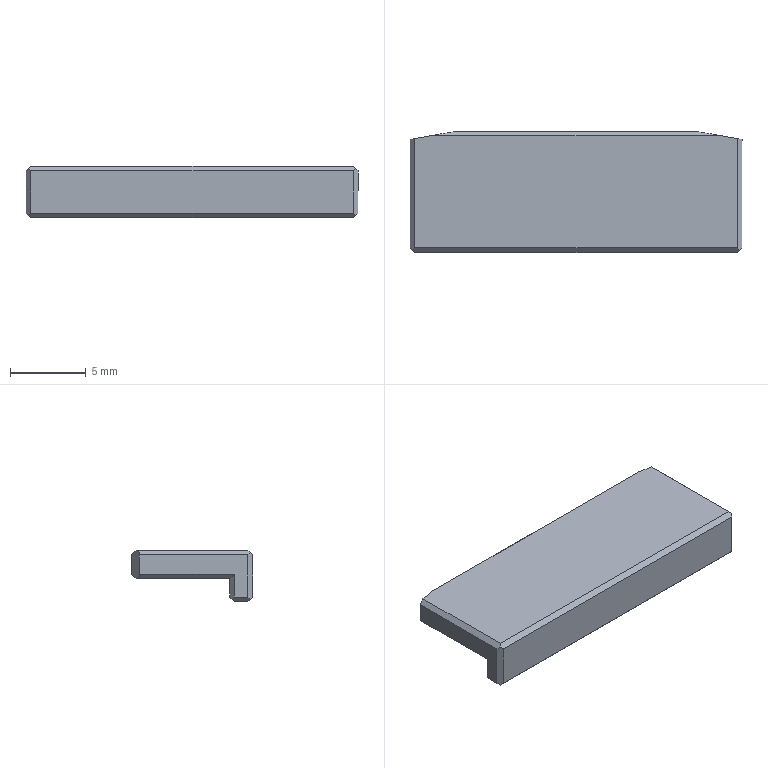Part | NX | 1 solid | 25 faces | box 21.95 x 8 x 3.38 mm | volume 370.348 mm3 | plane 25
STEP:
#1=CARTESIAN_POINT('',(-34.76,-62.629,7.853));
#2=VERTEX_POINT('',#1);
#3=CARTESIAN_POINT('',(-34.76,-56.605,7.853));
#4=VERTEX_POINT('',#3);
#5=CARTESIAN_POINT('',(-34.76,-59.529,7.853));
#6=DIRECTION('',(0.,1.,0.));
#7=VECTOR('',#6,1000.);
#8=LINE('',#5,#7);
#9=EDGE_CURVE('',#2,#4,#8,.T.);
#10=ORIENTED_EDGE('',*,*,#9,.T.);
#11=CARTESIAN_POINT('',(-33.762,-56.429,7.853));
#12=VERTEX_POINT('',#11);
#13=CARTESIAN_POINT('',(-22.513,-54.446,7.853));
#14=DIRECTION('',(0.9848,0.1736,0.));
#15=VECTOR('',#14,1000.);
#16=LINE('',#13,#15);
#17=EDGE_CURVE('',#4,#12,#16,.T.);
#18=ORIENTED_EDGE('',*,*,#17,.T.);
#19=CARTESIAN_POINT('',(-14.409,-56.429,7.853));
#20=VERTEX_POINT('',#19);
#21=CARTESIAN_POINT('',(-22.513,-56.429,7.853));
#22=DIRECTION('',(1.,0.,0.));
#23=VECTOR('',#22,1000.);
#24=LINE('',#21,#23);
#25=EDGE_CURVE('',#12,#20,#24,.T.);
#26=ORIENTED_EDGE('',*,*,#25,.T.);
#27=CARTESIAN_POINT('',(-13.41,-56.605,7.853));
#28=VERTEX_POINT('',#27);
#29=CARTESIAN_POINT('',(-22.513,-55.,7.853));
#30=DIRECTION('',(0.9848,-0.1736,0.));
#31=VECTOR('',#30,1000.);
#32=LINE('',#29,#31);
#33=EDGE_CURVE('',#20,#28,#32,.T.);
#34=ORIENTED_EDGE('',*,*,#33,.T.);
#35=CARTESIAN_POINT('',(-13.41,-62.629,7.853));
#36=VERTEX_POINT('',#35);
#37=CARTESIAN_POINT('',(-13.41,-59.643,7.853));
#38=DIRECTION('',(0.,-1.,0.));
#39=VECTOR('',#38,1000.);
#40=LINE('',#37,#39);
#41=EDGE_CURVE('',#28,#36,#40,.T.);
#42=ORIENTED_EDGE('',*,*,#41,.T.);
#43=CARTESIAN_POINT('',(-22.513,-62.629,7.853));
#44=DIRECTION('',(1.,0.,0.));
#45=VECTOR('',#44,1000.);
#46=LINE('',#43,#45);
#47=EDGE_CURVE('',#2,#36,#46,.T.);
#48=ORIENTED_EDGE('',*,*,#47,.F.);
#49=EDGE_LOOP('',(#10,#18,#26,#34,#42,#48));
#50=FACE_BOUND('',#49,.T.);
#51=CARTESIAN_POINT('',(-32.11,-63.129,7.853));
#52=DIRECTION('',(0.,0.,-1.));
#53=DIRECTION('',(0.,-1.,0.));
#54=AXIS2_PLACEMENT_3D('',#51,#52,#53);
#55=PLANE('',#54);
#56=ADVANCED_FACE('',(#50),#55,.T.);
#57=CARTESIAN_POINT('',(-35.06,-62.929,6.653));
#58=VERTEX_POINT('',#57);
#59=CARTESIAN_POINT('',(-35.06,-62.929,8.153));
#60=VERTEX_POINT('',#59);
#61=CARTESIAN_POINT('',(-35.06,-62.929,7.253));
#62=DIRECTION('',(0.,0.,1.));
#63=VECTOR('',#62,1000.);
#64=LINE('',#61,#63);
#65=EDGE_CURVE('',#58,#60,#64,.T.);
#66=ORIENTED_EDGE('',*,*,#65,.F.);
#67=CARTESIAN_POINT('',(-35.06,-63.829,6.653));
#68=VERTEX_POINT('',#67);
#69=CARTESIAN_POINT('',(-35.06,-63.379,6.653));
#70=DIRECTION('',(0.,1.,0.));
#71=VECTOR('',#70,1000.);
#72=LINE('',#69,#71);
#73=EDGE_CURVE('',#68,#58,#72,.T.);
#74=ORIENTED_EDGE('',*,*,#73,.F.);
#75=CARTESIAN_POINT('',(-35.06,-63.829,9.433));
#76=VERTEX_POINT('',#75);
#77=CARTESIAN_POINT('',(-35.06,-63.829,8.193));
#78=DIRECTION('',(0.,0.,-1.));
#79=VECTOR('',#78,1000.);
#80=LINE('',#77,#79);
#81=EDGE_CURVE('',#76,#68,#80,.T.);
#82=ORIENTED_EDGE('',*,*,#81,.F.);
#83=CARTESIAN_POINT('',(-35.06,-56.658,9.433));
#84=VERTEX_POINT('',#83);
#85=CARTESIAN_POINT('',(-35.06,-60.279,9.433));
#86=DIRECTION('',(0.,-1.,0.));
#87=VECTOR('',#86,1000.);
#88=LINE('',#85,#87);
#89=EDGE_CURVE('',#84,#76,#88,.T.);
#90=ORIENTED_EDGE('',*,*,#89,.F.);
#91=CARTESIAN_POINT('',(-35.06,-56.658,8.153));
#92=VERTEX_POINT('',#91);
#93=CARTESIAN_POINT('',(-35.06,-56.658,8.793));
#94=DIRECTION('',(0.,0.,-1.));
#95=VECTOR('',#94,1000.);
#96=LINE('',#93,#95);
#97=EDGE_CURVE('',#84,#92,#96,.T.);
#98=ORIENTED_EDGE('',*,*,#97,.T.);
#99=CARTESIAN_POINT('',(-35.06,-59.529,8.153));
#100=DIRECTION('',(0.,1.,0.));
#101=VECTOR('',#100,1000.);
#102=LINE('',#99,#101);
#103=EDGE_CURVE('',#60,#92,#102,.T.);
#104=ORIENTED_EDGE('',*,*,#103,.F.);
#105=EDGE_LOOP('',(#66,#74,#82,#90,#98,#104));
#106=FACE_BOUND('',#105,.T.);
#107=CARTESIAN_POINT('',(-35.06,-63.129,9.253));
#108=DIRECTION('',(-1.,0.,0.));
#109=DIRECTION('',(0.,0.,1.));
#110=AXIS2_PLACEMENT_3D('',#107,#108,#109);
#111=PLANE('',#110);
#112=ADVANCED_FACE('',(#106),#111,.T.);
#113=CARTESIAN_POINT('',(-34.76,-56.605,9.733));
#114=VERTEX_POINT('',#113);
#115=CARTESIAN_POINT('',(-34.76,-63.829,9.733));
#116=VERTEX_POINT('',#115);
#117=CARTESIAN_POINT('',(-34.76,-60.279,9.733));
#118=DIRECTION('',(0.,-1.,0.));
#119=VECTOR('',#118,1000.);
#120=LINE('',#117,#119);
#121=EDGE_CURVE('',#114,#116,#120,.T.);
#122=ORIENTED_EDGE('',*,*,#121,.T.);
#123=CARTESIAN_POINT('',(-13.41,-63.829,9.733));
#124=VERTEX_POINT('',#123);
#125=CARTESIAN_POINT('',(-24.085,-63.829,9.733));
#126=DIRECTION('',(-1.,0.,0.));
#127=VECTOR('',#126,1000.);
#128=LINE('',#125,#127);
#129=EDGE_CURVE('',#124,#116,#128,.T.);
#130=ORIENTED_EDGE('',*,*,#129,.F.);
#131=CARTESIAN_POINT('',(-13.41,-56.605,9.733));
#132=VERTEX_POINT('',#131);
#133=CARTESIAN_POINT('',(-13.41,-60.243,9.733));
#134=DIRECTION('',(0.,-1.,0.));
#135=VECTOR('',#134,1000.);
#136=LINE('',#133,#135);
#137=EDGE_CURVE('',#132,#124,#136,.T.);
#138=ORIENTED_EDGE('',*,*,#137,.F.);
#139=CARTESIAN_POINT('',(-14.409,-56.429,9.733));
#140=VERTEX_POINT('',#139);
#141=CARTESIAN_POINT('',(-22.513,-55.,9.733));
#142=DIRECTION('',(-0.9848,0.1736,0.));
#143=VECTOR('',#142,1000.);
#144=LINE('',#141,#143);
#145=EDGE_CURVE('',#132,#140,#144,.T.);
#146=ORIENTED_EDGE('',*,*,#145,.T.);
#147=CARTESIAN_POINT('',(-33.762,-56.429,9.733));
#148=VERTEX_POINT('',#147);
#149=CARTESIAN_POINT('',(-22.513,-56.429,9.733));
#150=DIRECTION('',(-1.,0.,0.));
#151=VECTOR('',#150,1000.);
#152=LINE('',#149,#151);
#153=EDGE_CURVE('',#140,#148,#152,.T.);
#154=ORIENTED_EDGE('',*,*,#153,.T.);
#155=CARTESIAN_POINT('',(-22.513,-54.446,9.733));
#156=DIRECTION('',(-0.9848,-0.1736,0.));
#157=VECTOR('',#156,1000.);
#158=LINE('',#155,#157);
#159=EDGE_CURVE('',#148,#114,#158,.T.);
#160=ORIENTED_EDGE('',*,*,#159,.T.);
#161=EDGE_LOOP('',(#122,#130,#138,#146,#154,#160));
#162=FACE_BOUND('',#161,.T.);
#163=CARTESIAN_POINT('',(-16.11,-63.129,9.733));
#164=DIRECTION('',(0.,0.,1.));
#165=DIRECTION('',(1.,0.,0.));
#166=AXIS2_PLACEMENT_3D('',#163,#164,#165);
#167=PLANE('',#166);
#168=ADVANCED_FACE('',(#162),#167,.T.);
#169=CARTESIAN_POINT('',(-13.11,-63.829,9.433));
#170=VERTEX_POINT('',#169);
#171=CARTESIAN_POINT('',(-13.11,-63.829,6.653));
#172=VERTEX_POINT('',#171);
#173=CARTESIAN_POINT('',(-13.11,-63.829,13.966));
#174=DIRECTION('',(0.,0.,-1.));
#175=VECTOR('',#174,1000.);
#176=LINE('',#173,#175);
#177=EDGE_CURVE('',#170,#172,#176,.T.);
#178=ORIENTED_EDGE('',*,*,#177,.T.);
#179=CARTESIAN_POINT('',(-13.11,-62.929,6.653));
#180=VERTEX_POINT('',#179);
#181=CARTESIAN_POINT('',(-13.11,-63.379,6.653));
#182=DIRECTION('',(0.,-1.,0.));
#183=VECTOR('',#182,1000.);
#184=LINE('',#181,#183);
#185=EDGE_CURVE('',#180,#172,#184,.T.);
#186=ORIENTED_EDGE('',*,*,#185,.F.);
#187=CARTESIAN_POINT('',(-13.11,-62.929,8.153));
#188=VERTEX_POINT('',#187);
#189=CARTESIAN_POINT('',(-13.11,-62.929,7.103));
#190=DIRECTION('',(0.,0.,-1.));
#191=VECTOR('',#190,1000.);
#192=LINE('',#189,#191);
#193=EDGE_CURVE('',#188,#180,#192,.T.);
#194=ORIENTED_EDGE('',*,*,#193,.F.);
#195=CARTESIAN_POINT('',(-13.11,-56.658,8.153));
#196=VERTEX_POINT('',#195);
#197=CARTESIAN_POINT('',(-13.11,-59.643,8.153));
#198=DIRECTION('',(0.,-1.,0.));
#199=VECTOR('',#198,1000.);
#200=LINE('',#197,#199);
#201=EDGE_CURVE('',#196,#188,#200,.T.);
#202=ORIENTED_EDGE('',*,*,#201,.F.);
#203=CARTESIAN_POINT('',(-13.11,-56.658,9.433));
#204=VERTEX_POINT('',#203);
#205=CARTESIAN_POINT('',(-13.11,-56.658,13.966));
#206=DIRECTION('',(0.,0.,1.));
#207=VECTOR('',#206,1000.);
#208=LINE('',#205,#207);
#209=EDGE_CURVE('',#196,#204,#208,.T.);
#210=ORIENTED_EDGE('',*,*,#209,.T.);
#211=CARTESIAN_POINT('',(-13.11,-60.243,9.433));
#212=DIRECTION('',(0.,-1.,0.));
#213=VECTOR('',#212,1000.);
#214=LINE('',#211,#213);
#215=EDGE_CURVE('',#204,#170,#214,.T.);
#216=ORIENTED_EDGE('',*,*,#215,.T.);
#217=EDGE_LOOP('',(#178,#186,#194,#202,#210,#216));
#218=FACE_BOUND('',#217,.T.);
#219=CARTESIAN_POINT('',(-13.11,-63.129,7.853));
#220=DIRECTION('',(1.,0.,0.));
#221=DIRECTION('',(0.,-1.,0.));
#222=AXIS2_PLACEMENT_3D('',#219,#220,#221);
#223=PLANE('',#222);
#224=ADVANCED_FACE('',(#218),#223,.T.);
#225=CARTESIAN_POINT('',(-34.76,-63.829,6.353));
#226=VERTEX_POINT('',#225);
#227=CARTESIAN_POINT('',(-34.76,-62.929,6.353));
#228=VERTEX_POINT('',#227);
#229=CARTESIAN_POINT('',(-34.76,-63.379,6.353));
#230=DIRECTION('',(0.,1.,0.));
#231=VECTOR('',#230,1000.);
#232=LINE('',#229,#231);
#233=EDGE_CURVE('',#226,#228,#232,.T.);
#234=ORIENTED_EDGE('',*,*,#233,.T.);
#235=CARTESIAN_POINT('',(-13.41,-62.929,6.353));
#236=VERTEX_POINT('',#235);
#237=CARTESIAN_POINT('',(-22.513,-62.929,6.353));
#238=DIRECTION('',(1.,0.,0.));
#239=VECTOR('',#238,1000.);
#240=LINE('',#237,#239);
#241=EDGE_CURVE('',#228,#236,#240,.T.);
#242=ORIENTED_EDGE('',*,*,#241,.T.);
#243=CARTESIAN_POINT('',(-13.41,-63.829,6.353));
#244=VERTEX_POINT('',#243);
#245=CARTESIAN_POINT('',(-13.41,-63.379,6.353));
#246=DIRECTION('',(0.,-1.,0.));
#247=VECTOR('',#246,1000.);
#248=LINE('',#245,#247);
#249=EDGE_CURVE('',#236,#244,#248,.T.);
#250=ORIENTED_EDGE('',*,*,#249,.T.);
#251=CARTESIAN_POINT('',(-22.513,-63.829,6.353));
#252=DIRECTION('',(-1.,0.,0.));
#253=VECTOR('',#252,1000.);
#254=LINE('',#251,#253);
#255=EDGE_CURVE('',#244,#226,#254,.T.);
#256=ORIENTED_EDGE('',*,*,#255,.T.);
#257=EDGE_LOOP('',(#234,#242,#250,#256));
#258=FACE_BOUND('',#257,.T.);
#259=CARTESIAN_POINT('',(-19.282,-63.809,6.353));
#260=DIRECTION('',(0.,0.,-1.));
#261=DIRECTION('',(0.,-1.,0.));
#262=AXIS2_PLACEMENT_3D('',#259,#260,#261);
#263=PLANE('',#262);
#264=ADVANCED_FACE('',(#258),#263,.T.);
#265=ORIENTED_EDGE('',*,*,#249,.F.);
#266=CARTESIAN_POINT('',(-13.26,-62.779,6.503));
#267=VERTEX_POINT('',#266);
#268=CARTESIAN_POINT('',(-13.61,-63.129,6.153));
#269=DIRECTION('',(-0.5774,-0.5774,-0.5774));
#270=VECTOR('',#269,1000.);
#271=LINE('',#268,#270);
#272=EDGE_CURVE('',#267,#236,#271,.T.);
#273=ORIENTED_EDGE('',*,*,#272,.F.);
#274=CARTESIAN_POINT('',(-22.513,-53.526,-2.75));
#275=DIRECTION('',(-0.5774,0.5774,-0.5774));
#276=VECTOR('',#275,1000.);
#277=LINE('',#274,#276);
#278=EDGE_CURVE('',#180,#267,#277,.T.);
#279=ORIENTED_EDGE('',*,*,#278,.F.);
#280=ORIENTED_EDGE('',*,*,#185,.T.);
#281=CARTESIAN_POINT('',(-13.26,-63.979,6.503));
#282=VERTEX_POINT('',#281);
#283=CARTESIAN_POINT('',(-22.513,-73.232,-2.75));
#284=DIRECTION('',(-0.5774,-0.5774,-0.5774));
#285=VECTOR('',#284,1000.);
#286=LINE('',#283,#285);
#287=EDGE_CURVE('',#172,#282,#286,.T.);
#288=ORIENTED_EDGE('',*,*,#287,.T.);
#289=CARTESIAN_POINT('',(-22.513,-54.726,-2.75));
#290=DIRECTION('',(0.5774,-0.5774,0.5774));
#291=VECTOR('',#290,1000.);
#292=LINE('',#289,#291);
#293=EDGE_CURVE('',#244,#282,#292,.T.);
#294=ORIENTED_EDGE('',*,*,#293,.F.);
#295=EDGE_LOOP('',(#265,#273,#279,#280,#288,#294));
#296=FACE_BOUND('',#295,.T.);
#297=CARTESIAN_POINT('',(-13.26,-63.379,6.503));
#298=DIRECTION('',(0.7071,0.,-0.7071));
#299=DIRECTION('',(0.,-1.,0.));
#300=AXIS2_PLACEMENT_3D('',#297,#298,#299);
#301=PLANE('',#300);
#302=ADVANCED_FACE('',(#296),#301,.T.);
#303=ORIENTED_EDGE('',*,*,#137,.T.);
#304=CARTESIAN_POINT('',(-13.26,-63.979,9.583));
#305=VERTEX_POINT('',#304);
#306=CARTESIAN_POINT('',(-22.513,-54.726,18.836));
#307=DIRECTION('',(0.5774,-0.5774,-0.5774));
#308=VECTOR('',#307,1000.);
#309=LINE('',#306,#308);
#310=EDGE_CURVE('',#124,#305,#309,.T.);
#311=ORIENTED_EDGE('',*,*,#310,.T.);
#312=CARTESIAN_POINT('',(-22.513,-73.232,18.836));
#313=DIRECTION('',(0.5774,0.5774,-0.5774));
#314=VECTOR('',#313,1000.);
#315=LINE('',#312,#314);
#316=EDGE_CURVE('',#305,#170,#315,.T.);
#317=ORIENTED_EDGE('',*,*,#316,.T.);
#318=ORIENTED_EDGE('',*,*,#215,.F.);
#319=CARTESIAN_POINT('',(-22.513,-55.,18.836));
#320=DIRECTION('',(-0.7017,0.1237,0.7017));
#321=VECTOR('',#320,1000.);
#322=LINE('',#319,#321);
#323=EDGE_CURVE('',#204,#132,#322,.T.);
#324=ORIENTED_EDGE('',*,*,#323,.T.);
#325=EDGE_LOOP('',(#303,#311,#317,#318,#324));
#326=FACE_BOUND('',#325,.T.);
#327=CARTESIAN_POINT('',(-13.26,-60.243,9.583));
#328=DIRECTION('',(-0.7071,0.,-0.7071));
#329=DIRECTION('',(-0.7071,0.,0.7071));
#330=AXIS2_PLACEMENT_3D('',#327,#328,#329);
#331=PLANE('',#330);
#332=ADVANCED_FACE('',(#326),#331,.F.);
#333=ORIENTED_EDGE('',*,*,#241,.F.);
#334=CARTESIAN_POINT('',(-34.91,-62.779,6.503));
#335=VERTEX_POINT('',#334);
#336=CARTESIAN_POINT('',(-22.513,-75.176,-5.894));
#337=DIRECTION('',(0.5774,-0.5774,-0.5774));
#338=VECTOR('',#337,1000.);
#339=LINE('',#336,#338);
#340=EDGE_CURVE('',#335,#228,#339,.T.);
#341=ORIENTED_EDGE('',*,*,#340,.F.);
#342=CARTESIAN_POINT('',(-34.76,-62.629,6.653));
#343=VERTEX_POINT('',#342);
#344=CARTESIAN_POINT('',(-35.26,-63.129,6.153));
#345=DIRECTION('',(0.5774,0.5774,0.5774));
#346=VECTOR('',#345,1000.);
#347=LINE('',#344,#346);
#348=EDGE_CURVE('',#335,#343,#347,.T.);
#349=ORIENTED_EDGE('',*,*,#348,.T.);
#350=CARTESIAN_POINT('',(-13.41,-62.629,6.653));
#351=VERTEX_POINT('',#350);
#352=CARTESIAN_POINT('',(-22.513,-62.629,6.653));
#353=DIRECTION('',(1.,0.,0.));
#354=VECTOR('',#353,1000.);
#355=LINE('',#352,#354);
#356=EDGE_CURVE('',#343,#351,#355,.T.);
#357=ORIENTED_EDGE('',*,*,#356,.T.);
#358=CARTESIAN_POINT('',(-22.513,-53.526,15.756));
#359=DIRECTION('',(0.5774,-0.5774,-0.5774));
#360=VECTOR('',#359,1000.);
#361=LINE('',#358,#360);
#362=EDGE_CURVE('',#351,#267,#361,.T.);
#363=ORIENTED_EDGE('',*,*,#362,.T.);
#364=ORIENTED_EDGE('',*,*,#272,.T.);
#365=EDGE_LOOP('',(#333,#341,#349,#357,#363,#364));
#366=FACE_BOUND('',#365,.T.);
#367=CARTESIAN_POINT('',(-24.11,-62.779,6.503));
#368=DIRECTION('',(0.,0.7071,-0.7071));
#369=DIRECTION('',(-1.,0.,0.));
#370=AXIS2_PLACEMENT_3D('',#367,#368,#369);
#371=PLANE('',#370);
#372=ADVANCED_FACE('',(#366),#371,.T.);
#373=CARTESIAN_POINT('',(-13.41,-64.129,6.653));
#374=VERTEX_POINT('',#373);
#375=CARTESIAN_POINT('',(-34.76,-64.129,6.653));
#376=VERTEX_POINT('',#375);
#377=CARTESIAN_POINT('',(-22.513,-64.129,6.653));
#378=DIRECTION('',(-1.,0.,0.));
#379=VECTOR('',#378,1000.);
#380=LINE('',#377,#379);
#381=EDGE_CURVE('',#374,#376,#380,.T.);
#382=ORIENTED_EDGE('',*,*,#381,.T.);
#383=CARTESIAN_POINT('',(-34.91,-63.979,6.503));
#384=VERTEX_POINT('',#383);
#385=CARTESIAN_POINT('',(-22.513,-76.376,18.9));
#386=DIRECTION('',(-0.5774,0.5774,-0.5774));
#387=VECTOR('',#386,1000.);
#388=LINE('',#385,#387);
#389=EDGE_CURVE('',#376,#384,#388,.T.);
#390=ORIENTED_EDGE('',*,*,#389,.T.);
#391=CARTESIAN_POINT('',(-22.513,-51.582,-5.894));
#392=DIRECTION('',(-0.5774,-0.5774,0.5774));
#393=VECTOR('',#392,1000.);
#394=LINE('',#391,#393);
#395=EDGE_CURVE('',#226,#384,#394,.T.);
#396=ORIENTED_EDGE('',*,*,#395,.F.);
#397=ORIENTED_EDGE('',*,*,#255,.F.);
#398=ORIENTED_EDGE('',*,*,#293,.T.);
#399=CARTESIAN_POINT('',(-22.513,-73.232,15.756));
#400=DIRECTION('',(0.5774,0.5774,-0.5774));
#401=VECTOR('',#400,1000.);
#402=LINE('',#399,#401);
#403=EDGE_CURVE('',#374,#282,#402,.T.);
#404=ORIENTED_EDGE('',*,*,#403,.F.);
#405=EDGE_LOOP('',(#382,#390,#396,#397,#398,#404));
#406=FACE_BOUND('',#405,.T.);
#407=CARTESIAN_POINT('',(-24.11,-63.979,6.503));
#408=DIRECTION('',(0.,-0.7071,-0.7071));
#409=DIRECTION('',(0.,-0.7071,0.7071));
#410=AXIS2_PLACEMENT_3D('',#407,#408,#409);
#411=PLANE('',#410);
#412=ADVANCED_FACE('',(#406),#411,.T.);
#413=ORIENTED_EDGE('',*,*,#41,.F.);
#414=CARTESIAN_POINT('',(-22.513,-55.,-1.25));
#415=DIRECTION('',(-0.7017,0.1237,-0.7017));
#416=VECTOR('',#415,1000.);
#417=LINE('',#414,#416);
#418=EDGE_CURVE('',#196,#28,#417,.T.);
#419=ORIENTED_EDGE('',*,*,#418,.F.);
#420=ORIENTED_EDGE('',*,*,#201,.T.);
#421=CARTESIAN_POINT('',(-22.513,-53.526,-1.25));
#422=DIRECTION('',(0.5774,-0.5774,0.5774));
#423=VECTOR('',#422,1000.);
#424=LINE('',#421,#423);
#425=EDGE_CURVE('',#36,#188,#424,.T.);
#426=ORIENTED_EDGE('',*,*,#425,.F.);
#427=EDGE_LOOP('',(#413,#419,#420,#426));
#428=FACE_BOUND('',#427,.T.);
#429=CARTESIAN_POINT('',(-13.26,-59.643,8.003));
#430=DIRECTION('',(0.7071,0.,-0.7071));
#431=DIRECTION('',(0.,-1.,0.));
#432=AXIS2_PLACEMENT_3D('',#429,#430,#431);
#433=PLANE('',#432);
#434=ADVANCED_FACE('',(#428),#433,.T.);
#435=ORIENTED_EDGE('',*,*,#89,.T.);
#436=CARTESIAN_POINT('',(-34.91,-63.979,9.583));
#437=VERTEX_POINT('',#436);
#438=CARTESIAN_POINT('',(-22.513,-76.376,21.98));
#439=DIRECTION('',(0.5774,-0.5774,0.5774));
#440=VECTOR('',#439,1000.);
#441=LINE('',#438,#440);
#442=EDGE_CURVE('',#76,#437,#441,.T.);
#443=ORIENTED_EDGE('',*,*,#442,.T.);
#444=CARTESIAN_POINT('',(-22.513,-51.582,21.98));
#445=DIRECTION('',(0.5774,0.5774,0.5774));
#446=VECTOR('',#445,1000.);
#447=LINE('',#444,#446);
#448=EDGE_CURVE('',#437,#116,#447,.T.);
#449=ORIENTED_EDGE('',*,*,#448,.T.);
#450=ORIENTED_EDGE('',*,*,#121,.F.);
#451=CARTESIAN_POINT('',(-22.513,-54.446,21.98));
#452=DIRECTION('',(0.7017,0.1237,0.7017));
#453=VECTOR('',#452,1000.);
#454=LINE('',#451,#453);
#455=EDGE_CURVE('',#84,#114,#454,.T.);
#456=ORIENTED_EDGE('',*,*,#455,.F.);
#457=EDGE_LOOP('',(#435,#443,#449,#450,#456));
#458=FACE_BOUND('',#457,.T.);
#459=CARTESIAN_POINT('',(-34.91,-60.279,9.583));
#460=DIRECTION('',(0.7071,0.,-0.7071));
#461=DIRECTION('',(0.,-1.,0.));
#462=AXIS2_PLACEMENT_3D('',#459,#460,#461);
#463=PLANE('',#462);
#464=ADVANCED_FACE('',(#458),#463,.F.);
#465=ORIENTED_EDGE('',*,*,#81,.T.);
#466=CARTESIAN_POINT('',(-22.513,-76.376,-5.894));
#467=DIRECTION('',(0.5774,-0.5774,-0.5774));
#468=VECTOR('',#467,1000.);
#469=LINE('',#466,#468);
#470=EDGE_CURVE('',#68,#384,#469,.T.);
#471=ORIENTED_EDGE('',*,*,#470,.T.);
#472=ORIENTED_EDGE('',*,*,#389,.F.);
#473=CARTESIAN_POINT('',(-34.76,-64.129,9.433));
#474=VERTEX_POINT('',#473);
#475=CARTESIAN_POINT('',(-34.76,-64.129,8.193));
#476=DIRECTION('',(0.,0.,-1.));
#477=VECTOR('',#476,1000.);
#478=LINE('',#475,#477);
#479=EDGE_CURVE('',#474,#376,#478,.T.);
#480=ORIENTED_EDGE('',*,*,#479,.F.);
#481=CARTESIAN_POINT('',(-22.513,-76.376,-2.814));
#482=DIRECTION('',(-0.5774,0.5774,0.5774));
#483=VECTOR('',#482,1000.);
#484=LINE('',#481,#483);
#485=EDGE_CURVE('',#474,#437,#484,.T.);
#486=ORIENTED_EDGE('',*,*,#485,.T.);
#487=ORIENTED_EDGE('',*,*,#442,.F.);
#488=EDGE_LOOP('',(#465,#471,#472,#480,#486,#487));
#489=FACE_BOUND('',#488,.T.);
#490=CARTESIAN_POINT('',(-34.91,-63.979,8.193));
#491=DIRECTION('',(0.7071,0.7071,0.));
#492=DIRECTION('',(0.,0.,-1.));
#493=AXIS2_PLACEMENT_3D('',#490,#491,#492);
#494=PLANE('',#493);
#495=ADVANCED_FACE('',(#489),#494,.F.);
#496=ORIENTED_EDGE('',*,*,#233,.F.);
#497=ORIENTED_EDGE('',*,*,#395,.T.);
#498=ORIENTED_EDGE('',*,*,#470,.F.);
#499=ORIENTED_EDGE('',*,*,#73,.T.);
#500=CARTESIAN_POINT('',(-35.26,-63.129,6.853));
#501=DIRECTION('',(0.5774,0.5774,-0.5774));
#502=VECTOR('',#501,1000.);
#503=LINE('',#500,#502);
#504=EDGE_CURVE('',#58,#335,#503,.T.);
#505=ORIENTED_EDGE('',*,*,#504,.T.);
#506=ORIENTED_EDGE('',*,*,#340,.T.);
#507=EDGE_LOOP('',(#496,#497,#498,#499,#505,#506));
#508=FACE_BOUND('',#507,.T.);
#509=CARTESIAN_POINT('',(-34.91,-63.379,6.503));
#510=DIRECTION('',(-0.7071,0.,-0.7071));
#511=DIRECTION('',(-0.7071,0.,0.7071));
#512=AXIS2_PLACEMENT_3D('',#509,#510,#511);
#513=PLANE('',#512);
#514=ADVANCED_FACE('',(#508),#513,.T.);
#515=ORIENTED_EDGE('',*,*,#65,.T.);
#516=CARTESIAN_POINT('',(-35.26,-63.129,8.353));
#517=DIRECTION('',(0.5774,0.5774,-0.5774));
#518=VECTOR('',#517,1000.);
#519=LINE('',#516,#518);
#520=EDGE_CURVE('',#60,#2,#519,.T.);
#521=ORIENTED_EDGE('',*,*,#520,.T.);
#522=CARTESIAN_POINT('',(-34.76,-62.629,7.253));
#523=DIRECTION('',(0.,0.,1.));
#524=VECTOR('',#523,1000.);
#525=LINE('',#522,#524);
#526=EDGE_CURVE('',#343,#2,#525,.T.);
#527=ORIENTED_EDGE('',*,*,#526,.F.);
#528=ORIENTED_EDGE('',*,*,#348,.F.);
#529=ORIENTED_EDGE('',*,*,#504,.F.);
#530=EDGE_LOOP('',(#515,#521,#527,#528,#529));
#531=FACE_BOUND('',#530,.T.);
#532=CARTESIAN_POINT('',(-34.91,-62.779,7.253));
#533=DIRECTION('',(0.7071,-0.7071,0.));
#534=DIRECTION('',(0.,0.,-1.));
#535=AXIS2_PLACEMENT_3D('',#532,#533,#534);
#536=PLANE('',#535);
#537=ADVANCED_FACE('',(#531),#536,.F.);
#538=ORIENTED_EDGE('',*,*,#9,.F.);
#539=ORIENTED_EDGE('',*,*,#520,.F.);
#540=ORIENTED_EDGE('',*,*,#103,.T.);
#541=CARTESIAN_POINT('',(-22.513,-54.446,-4.394));
#542=DIRECTION('',(0.7017,0.1237,-0.7017));
#543=VECTOR('',#542,1000.);
#544=LINE('',#541,#543);
#545=EDGE_CURVE('',#92,#4,#544,.T.);
#546=ORIENTED_EDGE('',*,*,#545,.T.);
#547=EDGE_LOOP('',(#538,#539,#540,#546));
#548=FACE_BOUND('',#547,.T.);
#549=CARTESIAN_POINT('',(-34.91,-59.529,8.003));
#550=DIRECTION('',(-0.7071,0.,-0.7071));
#551=DIRECTION('',(-0.7071,0.,0.7071));
#552=AXIS2_PLACEMENT_3D('',#549,#550,#551);
#553=PLANE('',#552);
#554=ADVANCED_FACE('',(#548),#553,.T.);
#555=CARTESIAN_POINT('',(-32.06,-56.129,9.433));
#556=VERTEX_POINT('',#555);
#557=CARTESIAN_POINT('',(-32.06,-56.129,8.153));
#558=VERTEX_POINT('',#557);
#559=CARTESIAN_POINT('',(-32.06,-56.129,8.793));
#560=DIRECTION('',(0.,0.,-1.));
#561=VECTOR('',#560,1000.);
#562=LINE('',#559,#561);
#563=EDGE_CURVE('',#556,#558,#562,.T.);
#564=ORIENTED_EDGE('',*,*,#563,.F.);
#565=CARTESIAN_POINT('',(-16.11,-56.129,9.433));
#566=VERTEX_POINT('',#565);
#567=CARTESIAN_POINT('',(-22.513,-56.129,9.433));
#568=DIRECTION('',(-1.,0.,0.));
#569=VECTOR('',#568,1000.);
#570=LINE('',#567,#569);
#571=EDGE_CURVE('',#566,#556,#570,.T.);
#572=ORIENTED_EDGE('',*,*,#571,.F.);
#573=CARTESIAN_POINT('',(-16.11,-56.129,8.153));
#574=VERTEX_POINT('',#573);
#575=CARTESIAN_POINT('',(-16.11,-56.129,13.966));
#576=DIRECTION('',(0.,0.,1.));
#577=VECTOR('',#576,1000.);
#578=LINE('',#575,#577);
#579=EDGE_CURVE('',#574,#566,#578,.T.);
#580=ORIENTED_EDGE('',*,*,#579,.F.);
#581=CARTESIAN_POINT('',(-22.513,-56.129,8.153));
#582=DIRECTION('',(1.,0.,0.));
#583=VECTOR('',#582,1000.);
#584=LINE('',#581,#583);
#585=EDGE_CURVE('',#558,#574,#584,.T.);
#586=ORIENTED_EDGE('',*,*,#585,.F.);
#587=EDGE_LOOP('',(#564,#572,#580,#586));
#588=FACE_BOUND('',#587,.T.);
#589=CARTESIAN_POINT('',(-22.513,-56.129,13.966));
#590=DIRECTION('',(0.,-1.,0.));
#591=DIRECTION('',(-1.,0.,0.));
#592=AXIS2_PLACEMENT_3D('',#589,#590,#591);
#593=PLANE('',#592);
#594=ADVANCED_FACE('',(#588),#593,.F.);
#595=ORIENTED_EDGE('',*,*,#579,.T.);
#596=CARTESIAN_POINT('',(-22.513,-55.,8.304));
#597=DIRECTION('',(-0.9703,0.1711,-0.1711));
#598=VECTOR('',#597,1000.);
#599=LINE('',#596,#598);
#600=EDGE_CURVE('',#140,#566,#599,.T.);
#601=ORIENTED_EDGE('',*,*,#600,.F.);
#602=ORIENTED_EDGE('',*,*,#145,.F.);
#603=ORIENTED_EDGE('',*,*,#323,.F.);
#604=ORIENTED_EDGE('',*,*,#209,.F.);
#605=ORIENTED_EDGE('',*,*,#418,.T.);
#606=ORIENTED_EDGE('',*,*,#33,.F.);
#607=CARTESIAN_POINT('',(-22.513,-55.,9.282));
#608=DIRECTION('',(0.9703,-0.1711,-0.1711));
#609=VECTOR('',#608,1000.);
#610=LINE('',#607,#609);
#611=EDGE_CURVE('',#574,#20,#610,.T.);
#612=ORIENTED_EDGE('',*,*,#611,.F.);
#613=EDGE_LOOP('',(#595,#601,#602,#603,#604,#605,#606,#612));
#614=FACE_BOUND('',#613,.T.);
#615=CARTESIAN_POINT('',(-14.61,-56.393,8.553));
#616=DIRECTION('',(-0.1736,-0.9848,0.));
#617=DIRECTION('',(-0.9848,0.1736,0.));
#618=AXIS2_PLACEMENT_3D('',#615,#616,#617);
#619=PLANE('',#618);
#620=ADVANCED_FACE('',(#614),#619,.F.);
#621=ORIENTED_EDGE('',*,*,#571,.T.);
#622=CARTESIAN_POINT('',(-22.513,-54.446,7.75));
#623=DIRECTION('',(0.9703,0.1711,-0.1711));
#624=VECTOR('',#623,1000.);
#625=LINE('',#622,#624);
#626=EDGE_CURVE('',#148,#556,#625,.T.);
#627=ORIENTED_EDGE('',*,*,#626,.F.);
#628=ORIENTED_EDGE('',*,*,#153,.F.);
#629=ORIENTED_EDGE('',*,*,#600,.T.);
#630=EDGE_LOOP('',(#621,#627,#628,#629));
#631=FACE_BOUND('',#630,.T.);
#632=CARTESIAN_POINT('',(-24.11,-56.279,9.583));
#633=DIRECTION('',(0.,-0.7071,-0.7071));
#634=DIRECTION('',(0.,-0.7071,0.7071));
#635=AXIS2_PLACEMENT_3D('',#632,#633,#634);
#636=PLANE('',#635);
#637=ADVANCED_FACE('',(#631),#636,.F.);
#638=ORIENTED_EDGE('',*,*,#25,.F.);
#639=CARTESIAN_POINT('',(-22.513,-54.446,9.837));
#640=DIRECTION('',(-0.9703,-0.1711,-0.1711));
#641=VECTOR('',#640,1000.);
#642=LINE('',#639,#641);
#643=EDGE_CURVE('',#558,#12,#642,.T.);
#644=ORIENTED_EDGE('',*,*,#643,.F.);
#645=ORIENTED_EDGE('',*,*,#585,.T.);
#646=ORIENTED_EDGE('',*,*,#611,.T.);
#647=EDGE_LOOP('',(#638,#644,#645,#646));
#648=FACE_BOUND('',#647,.T.);
#649=CARTESIAN_POINT('',(-24.11,-56.279,8.003));
#650=DIRECTION('',(0.,-0.7071,0.7071));
#651=DIRECTION('',(-1.,0.,0.));
#652=AXIS2_PLACEMENT_3D('',#649,#650,#651);
#653=PLANE('',#652);
#654=ADVANCED_FACE('',(#648),#653,.F.);
#655=ORIENTED_EDGE('',*,*,#563,.T.);
#656=ORIENTED_EDGE('',*,*,#643,.T.);
#657=ORIENTED_EDGE('',*,*,#17,.F.);
#658=ORIENTED_EDGE('',*,*,#545,.F.);
#659=ORIENTED_EDGE('',*,*,#97,.F.);
#660=ORIENTED_EDGE('',*,*,#455,.T.);
#661=ORIENTED_EDGE('',*,*,#159,.F.);
#662=ORIENTED_EDGE('',*,*,#626,.T.);
#663=EDGE_LOOP('',(#655,#656,#657,#658,#659,#660,#661,#662));
#664=FACE_BOUND('',#663,.T.);
#665=CARTESIAN_POINT('',(-33.56,-56.393,8.793));
#666=DIRECTION('',(0.1736,-0.9848,0.));
#667=DIRECTION('',(0.,0.,-1.));
#668=AXIS2_PLACEMENT_3D('',#665,#666,#667);
#669=PLANE('',#668);
#670=ADVANCED_FACE('',(#664),#669,.F.);
#671=CARTESIAN_POINT('',(-13.41,-64.129,9.433));
#672=VERTEX_POINT('',#671);
#673=CARTESIAN_POINT('',(-24.085,-64.129,9.433));
#674=DIRECTION('',(-1.,0.,0.));
#675=VECTOR('',#674,1000.);
#676=LINE('',#673,#675);
#677=EDGE_CURVE('',#672,#474,#676,.T.);
#678=ORIENTED_EDGE('',*,*,#677,.T.);
#679=ORIENTED_EDGE('',*,*,#479,.T.);
#680=ORIENTED_EDGE('',*,*,#381,.F.);
#681=CARTESIAN_POINT('',(-13.41,-64.129,13.966));
#682=DIRECTION('',(0.,0.,-1.));
#683=VECTOR('',#682,1000.);
#684=LINE('',#681,#683);
#685=EDGE_CURVE('',#672,#374,#684,.T.);
#686=ORIENTED_EDGE('',*,*,#685,.F.);
#687=EDGE_LOOP('',(#678,#679,#680,#686));
#688=FACE_BOUND('',#687,.T.);
#689=CARTESIAN_POINT('',(-22.513,-64.129,13.966));
#690=DIRECTION('',(0.,-1.,0.));
#691=DIRECTION('',(-1.,0.,0.));
#692=AXIS2_PLACEMENT_3D('',#689,#690,#691);
#693=PLANE('',#692);
#694=ADVANCED_FACE('',(#688),#693,.T.);
#695=ORIENTED_EDGE('',*,*,#526,.T.);
#696=ORIENTED_EDGE('',*,*,#47,.T.);
#697=CARTESIAN_POINT('',(-13.41,-62.629,7.103));
#698=DIRECTION('',(0.,0.,-1.));
#699=VECTOR('',#698,1000.);
#700=LINE('',#697,#699);
#701=EDGE_CURVE('',#36,#351,#700,.T.);
#702=ORIENTED_EDGE('',*,*,#701,.T.);
#703=ORIENTED_EDGE('',*,*,#356,.F.);
#704=EDGE_LOOP('',(#695,#696,#702,#703));
#705=FACE_BOUND('',#704,.T.);
#706=CARTESIAN_POINT('',(-16.21,-62.629,7.853));
#707=DIRECTION('',(0.,1.,0.));
#708=DIRECTION('',(1.,0.,0.));
#709=AXIS2_PLACEMENT_3D('',#706,#707,#708);
#710=PLANE('',#709);
#711=ADVANCED_FACE('',(#705),#710,.T.);
#712=ORIENTED_EDGE('',*,*,#316,.F.);
#713=CARTESIAN_POINT('',(-22.513,-73.232,0.3302));
#714=DIRECTION('',(-0.5774,-0.5774,-0.5774));
#715=VECTOR('',#714,1000.);
#716=LINE('',#713,#715);
#717=EDGE_CURVE('',#305,#672,#716,.T.);
#718=ORIENTED_EDGE('',*,*,#717,.T.);
#719=ORIENTED_EDGE('',*,*,#685,.T.);
#720=ORIENTED_EDGE('',*,*,#403,.T.);
#721=ORIENTED_EDGE('',*,*,#287,.F.);
#722=ORIENTED_EDGE('',*,*,#177,.F.);
#723=EDGE_LOOP('',(#712,#718,#719,#720,#721,#722));
#724=FACE_BOUND('',#723,.T.);
#725=CARTESIAN_POINT('',(-13.26,-63.979,8.053));
#726=DIRECTION('',(-0.7071,0.7071,0.));
#727=DIRECTION('',(0.,0.,1.));
#728=AXIS2_PLACEMENT_3D('',#725,#726,#727);
#729=PLANE('',#728);
#730=ADVANCED_FACE('',(#724),#729,.F.);
#731=ORIENTED_EDGE('',*,*,#701,.F.);
#732=ORIENTED_EDGE('',*,*,#425,.T.);
#733=ORIENTED_EDGE('',*,*,#193,.T.);
#734=ORIENTED_EDGE('',*,*,#278,.T.);
#735=ORIENTED_EDGE('',*,*,#362,.F.);
#736=EDGE_LOOP('',(#731,#732,#733,#734,#735));
#737=FACE_BOUND('',#736,.T.);
#738=CARTESIAN_POINT('',(-13.26,-62.779,7.103));
#739=DIRECTION('',(0.7071,0.7071,0.));
#740=DIRECTION('',(0.,0.,-1.));
#741=AXIS2_PLACEMENT_3D('',#738,#739,#740);
#742=PLANE('',#741);
#743=ADVANCED_FACE('',(#737),#742,.T.);
#744=ORIENTED_EDGE('',*,*,#677,.F.);
#745=ORIENTED_EDGE('',*,*,#717,.F.);
#746=ORIENTED_EDGE('',*,*,#310,.F.);
#747=ORIENTED_EDGE('',*,*,#129,.T.);
#748=ORIENTED_EDGE('',*,*,#448,.F.);
#749=ORIENTED_EDGE('',*,*,#485,.F.);
#750=EDGE_LOOP('',(#744,#745,#746,#747,#748,#749));
#751=FACE_BOUND('',#750,.T.);
#752=CARTESIAN_POINT('',(-24.085,-63.979,9.583));
#753=DIRECTION('',(0.,-0.7071,0.7071));
#754=DIRECTION('',(-1.,0.,0.));
#755=AXIS2_PLACEMENT_3D('',#752,#753,#754);
#756=PLANE('',#755);
#757=ADVANCED_FACE('',(#751),#756,.T.);
#758=CLOSED_SHELL('',(#56,#112,#168,#224,#264,#302,#332,#372,#412,#434,#464,#495,#514,#537,#554,#594,#620,#637,#654,#670,#694,#711,#730,#743,#757));
#759=MANIFOLD_SOLID_BREP('',#758);
#760=(LENGTH_UNIT()NAMED_UNIT(*)SI_UNIT(.MILLI.,.METRE.));
#761=UNCERTAINTY_MEASURE_WITH_UNIT(LENGTH_MEASURE(0.00001),#760,'','');
#762=(NAMED_UNIT(*)PLANE_ANGLE_UNIT()SI_UNIT($,.RADIAN.));
#763=(NAMED_UNIT(*)SI_UNIT($,.STERADIAN.)SOLID_ANGLE_UNIT());
#764=(GEOMETRIC_REPRESENTATION_CONTEXT(3)GLOBAL_UNCERTAINTY_ASSIGNED_CONTEXT((#761))GLOBAL_UNIT_ASSIGNED_CONTEXT((#760,#762,#763))REPRESENTATION_CONTEXT('',''));
#765=ADVANCED_BREP_SHAPE_REPRESENTATION('',(#759),#764);